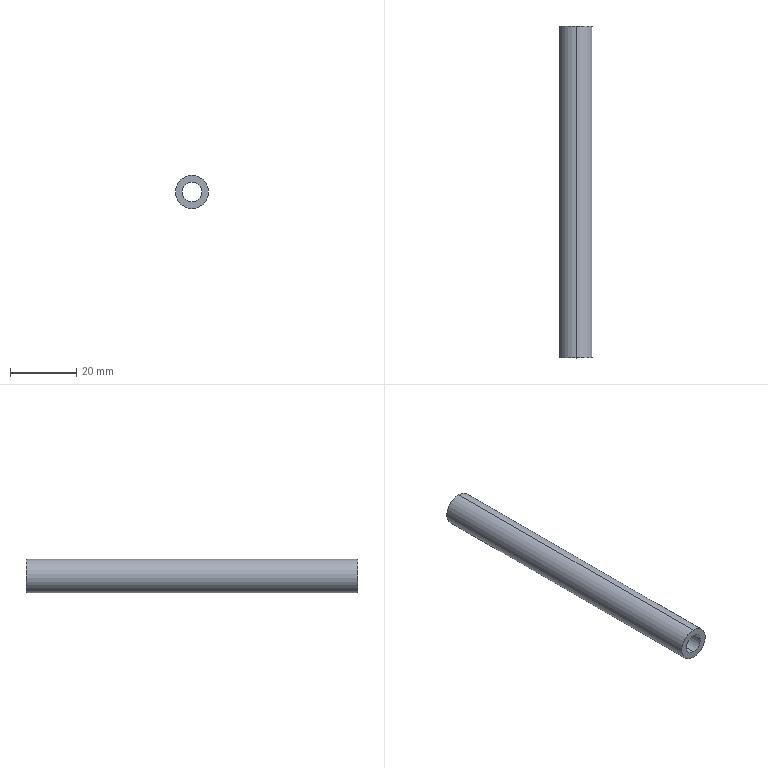Part | SolidWorks | features Extrusion 1 | 1 solid | 6 faces | box 10 x 100 x 10 mm | volume 5027 mm3 | cylinder 4 | plane 2 | commonest cylinder face diameters 6 x2 10 x2
STEP:
#1=CARTESIAN_POINT('',(0.,100.,-3.));
#2=VERTEX_POINT('',#1);
#3=CARTESIAN_POINT('',(0.,100.,3.));
#4=VERTEX_POINT('',#3);
#5=CARTESIAN_POINT('',(0.,100.,0.));
#6=DIRECTION('',(0.,1.,0.));
#7=DIRECTION('',(0.,0.,1.));
#8=AXIS2_PLACEMENT_3D('',#5,#6,#7);
#9=CIRCLE('',#8,3.);
#10=EDGE_CURVE('',#2,#4,#9,.T.);
#11=ORIENTED_EDGE('',*,*,#10,.T.);
#12=CARTESIAN_POINT('',(0.,0.,3.));
#13=VERTEX_POINT('',#12);
#14=CARTESIAN_POINT('',(0.,100.,3.));
#15=DIRECTION('',(0.,-1.,0.));
#16=VECTOR('',#15,1000.);
#17=LINE('',#14,#16);
#18=EDGE_CURVE('',#4,#13,#17,.T.);
#19=ORIENTED_EDGE('',*,*,#18,.T.);
#20=CARTESIAN_POINT('',(0.,0.,-3.));
#21=VERTEX_POINT('',#20);
#22=CARTESIAN_POINT('',(0.,0.,0.));
#23=DIRECTION('',(0.,1.,0.));
#24=DIRECTION('',(0.,0.,1.));
#25=AXIS2_PLACEMENT_3D('',#22,#23,#24);
#26=CIRCLE('',#25,3.);
#27=EDGE_CURVE('',#21,#13,#26,.T.);
#28=ORIENTED_EDGE('',*,*,#27,.F.);
#29=CARTESIAN_POINT('',(0.,100.,-3.));
#30=DIRECTION('',(0.,-1.,0.));
#31=VECTOR('',#30,1000.);
#32=LINE('',#29,#31);
#33=EDGE_CURVE('',#2,#21,#32,.T.);
#34=ORIENTED_EDGE('',*,*,#33,.F.);
#35=EDGE_LOOP('',(#11,#19,#28,#34));
#36=FACE_OUTER_BOUND('',#35,.T.);
#37=CARTESIAN_POINT('',(0.,100.,0.));
#38=DIRECTION('',(0.,-1.,0.));
#39=DIRECTION('',(0.,0.,-1.));
#40=AXIS2_PLACEMENT_3D('',#37,#38,#39);
#41=CYLINDRICAL_SURFACE('',#40,3.);
#42=ADVANCED_FACE('',(#36),#41,.F.);
#43=CARTESIAN_POINT('',(0.,100.,5.));
#44=VERTEX_POINT('',#43);
#45=CARTESIAN_POINT('',(0.,100.,-5.));
#46=VERTEX_POINT('',#45);
#47=CARTESIAN_POINT('',(0.,100.,0.));
#48=DIRECTION('',(0.,1.,0.));
#49=DIRECTION('',(0.,0.,1.));
#50=AXIS2_PLACEMENT_3D('',#47,#48,#49);
#51=CIRCLE('',#50,5.);
#52=EDGE_CURVE('',#44,#46,#51,.T.);
#53=ORIENTED_EDGE('',*,*,#52,.F.);
#54=CARTESIAN_POINT('',(0.,0.,5.));
#55=VERTEX_POINT('',#54);
#56=CARTESIAN_POINT('',(0.,100.,5.));
#57=DIRECTION('',(0.,-1.,0.));
#58=VECTOR('',#57,1000.);
#59=LINE('',#56,#58);
#60=EDGE_CURVE('',#44,#55,#59,.T.);
#61=ORIENTED_EDGE('',*,*,#60,.T.);
#62=CARTESIAN_POINT('',(0.,0.,-5.));
#63=VERTEX_POINT('',#62);
#64=CARTESIAN_POINT('',(0.,0.,0.));
#65=DIRECTION('',(0.,1.,0.));
#66=DIRECTION('',(0.,0.,1.));
#67=AXIS2_PLACEMENT_3D('',#64,#65,#66);
#68=CIRCLE('',#67,5.);
#69=EDGE_CURVE('',#55,#63,#68,.T.);
#70=ORIENTED_EDGE('',*,*,#69,.T.);
#71=CARTESIAN_POINT('',(0.,100.,-5.));
#72=DIRECTION('',(0.,-1.,0.));
#73=VECTOR('',#72,1000.);
#74=LINE('',#71,#73);
#75=EDGE_CURVE('',#46,#63,#74,.T.);
#76=ORIENTED_EDGE('',*,*,#75,.F.);
#77=EDGE_LOOP('',(#53,#61,#70,#76));
#78=FACE_OUTER_BOUND('',#77,.T.);
#79=CARTESIAN_POINT('',(0.,100.,0.));
#80=DIRECTION('',(0.,-1.,0.));
#81=DIRECTION('',(0.,0.,-1.));
#82=AXIS2_PLACEMENT_3D('',#79,#80,#81);
#83=CYLINDRICAL_SURFACE('',#82,5.);
#84=ADVANCED_FACE('',(#78),#83,.T.);
#85=CARTESIAN_POINT('',(0.,100.,0.));
#86=DIRECTION('',(0.,1.,0.));
#87=DIRECTION('',(0.,0.,1.));
#88=AXIS2_PLACEMENT_3D('',#85,#86,#87);
#89=CIRCLE('',#88,5.);
#90=EDGE_CURVE('',#46,#44,#89,.T.);
#91=ORIENTED_EDGE('',*,*,#90,.T.);
#92=ORIENTED_EDGE('',*,*,#52,.T.);
#93=EDGE_LOOP('',(#91,#92));
#94=FACE_OUTER_BOUND('',#93,.T.);
#95=ORIENTED_EDGE('',*,*,#10,.F.);
#96=CARTESIAN_POINT('',(0.,100.,0.));
#97=DIRECTION('',(0.,1.,0.));
#98=DIRECTION('',(0.,0.,1.));
#99=AXIS2_PLACEMENT_3D('',#96,#97,#98);
#100=CIRCLE('',#99,3.);
#101=EDGE_CURVE('',#4,#2,#100,.T.);
#102=ORIENTED_EDGE('',*,*,#101,.F.);
#103=EDGE_LOOP('',(#95,#102));
#104=FACE_BOUND('',#103,.T.);
#105=CARTESIAN_POINT('',(0.,100.,0.));
#106=DIRECTION('',(0.,1.,0.));
#107=DIRECTION('',(0.,0.,1.));
#108=AXIS2_PLACEMENT_3D('',#105,#106,#107);
#109=PLANE('',#108);
#110=ADVANCED_FACE('',(#94,#104),#109,.T.);
#111=CARTESIAN_POINT('',(0.,0.,0.));
#112=DIRECTION('',(0.,1.,0.));
#113=DIRECTION('',(0.,0.,1.));
#114=AXIS2_PLACEMENT_3D('',#111,#112,#113);
#115=CIRCLE('',#114,5.);
#116=EDGE_CURVE('',#63,#55,#115,.T.);
#117=ORIENTED_EDGE('',*,*,#116,.F.);
#118=ORIENTED_EDGE('',*,*,#69,.F.);
#119=EDGE_LOOP('',(#117,#118));
#120=FACE_OUTER_BOUND('',#119,.T.);
#121=ORIENTED_EDGE('',*,*,#27,.T.);
#122=CARTESIAN_POINT('',(0.,0.,0.));
#123=DIRECTION('',(0.,1.,0.));
#124=DIRECTION('',(0.,0.,1.));
#125=AXIS2_PLACEMENT_3D('',#122,#123,#124);
#126=CIRCLE('',#125,3.);
#127=EDGE_CURVE('',#13,#21,#126,.T.);
#128=ORIENTED_EDGE('',*,*,#127,.T.);
#129=EDGE_LOOP('',(#121,#128));
#130=FACE_BOUND('',#129,.T.);
#131=CARTESIAN_POINT('',(0.,0.,0.));
#132=DIRECTION('',(0.,1.,0.));
#133=DIRECTION('',(0.,0.,1.));
#134=AXIS2_PLACEMENT_3D('',#131,#132,#133);
#135=PLANE('',#134);
#136=ADVANCED_FACE('',(#120,#130),#135,.F.);
#137=ORIENTED_EDGE('',*,*,#60,.F.);
#138=ORIENTED_EDGE('',*,*,#90,.F.);
#139=ORIENTED_EDGE('',*,*,#75,.T.);
#140=ORIENTED_EDGE('',*,*,#116,.T.);
#141=EDGE_LOOP('',(#137,#138,#139,#140));
#142=FACE_OUTER_BOUND('',#141,.T.);
#143=CARTESIAN_POINT('',(0.,100.,0.));
#144=DIRECTION('',(0.,-1.,0.));
#145=DIRECTION('',(0.,0.,-1.));
#146=AXIS2_PLACEMENT_3D('',#143,#144,#145);
#147=CYLINDRICAL_SURFACE('',#146,5.);
#148=ADVANCED_FACE('',(#142),#147,.T.);
#149=ORIENTED_EDGE('',*,*,#18,.F.);
#150=ORIENTED_EDGE('',*,*,#101,.T.);
#151=ORIENTED_EDGE('',*,*,#33,.T.);
#152=ORIENTED_EDGE('',*,*,#127,.F.);
#153=EDGE_LOOP('',(#149,#150,#151,#152));
#154=FACE_OUTER_BOUND('',#153,.T.);
#155=CARTESIAN_POINT('',(0.,100.,0.));
#156=DIRECTION('',(0.,-1.,0.));
#157=DIRECTION('',(0.,0.,-1.));
#158=AXIS2_PLACEMENT_3D('',#155,#156,#157);
#159=CYLINDRICAL_SURFACE('',#158,3.);
#160=ADVANCED_FACE('',(#154),#159,.F.);
#161=CLOSED_SHELL('',(#42,#84,#110,#136,#148,#160));
#162=MANIFOLD_SOLID_BREP('',#161);
#163=CARTESIAN_POINT('',(0.,0.,0.));
#164=DIRECTION('',(0.,0.,1.));
#165=DIRECTION('',(1.,0.,0.));
#166=AXIS2_PLACEMENT_3D('',#163,#164,#165);
#167=(LENGTH_UNIT()NAMED_UNIT(*)SI_UNIT(.MILLI.,.METRE.));
#168=UNCERTAINTY_MEASURE_WITH_UNIT(LENGTH_MEASURE(0.00001),#167,'','');
#169=(NAMED_UNIT(*)PLANE_ANGLE_UNIT()SI_UNIT($,.RADIAN.));
#170=(NAMED_UNIT(*)SI_UNIT($,.STERADIAN.)SOLID_ANGLE_UNIT());
#171=(GEOMETRIC_REPRESENTATION_CONTEXT(3)GLOBAL_UNCERTAINTY_ASSIGNED_CONTEXT((#168))GLOBAL_UNIT_ASSIGNED_CONTEXT((#167,#169,#170))REPRESENTATION_CONTEXT('',''));
#172=ADVANCED_BREP_SHAPE_REPRESENTATION('',(#162,#166),#171);